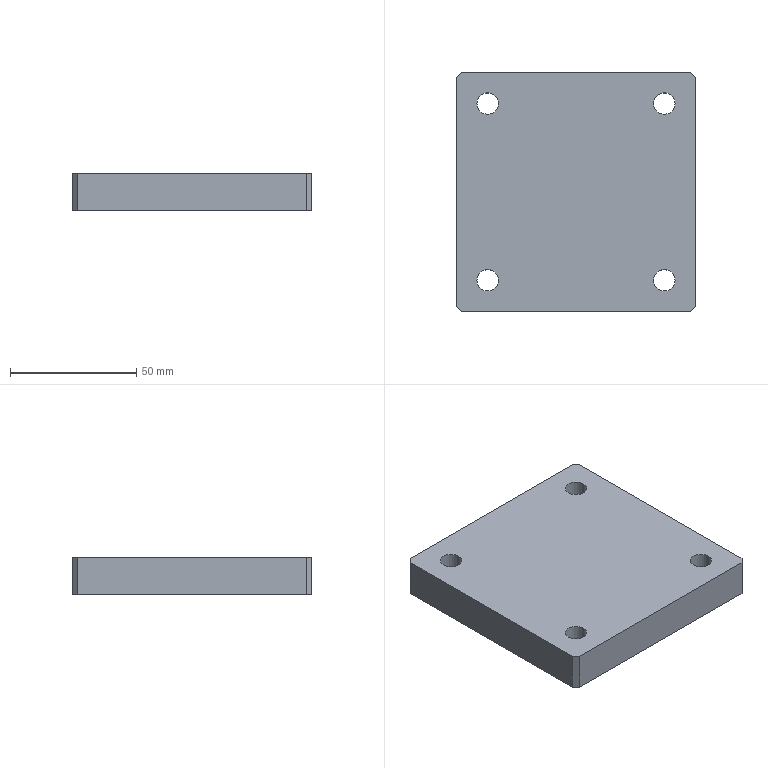Part | STEP file | ASND-0110-E63-HLTP01-005 | 1 solid | 18 faces | box 95 x 95 x 15 mm | volume 131850 mm3 | plane 10 | cylinder 8 | commonest cylinder face diameters 8.5 x8
STEP:
#1=CARTESIAN_POINT('',(0.,0.,0.));
#2=DIRECTION('',(0.,0.,1.));
#3=DIRECTION('',(1.,0.,0.));
#4=AXIS2_PLACEMENT_3D('',#1,#2,#3);
#5=CARTESIAN_POINT('',(16.75,82.5,0.));
#6=VERTEX_POINT('',#5);
#7=CARTESIAN_POINT('',(16.75,82.5,15.));
#8=VERTEX_POINT('',#7);
#9=CARTESIAN_POINT('',(16.75,82.5,15.));
#10=DIRECTION('',(0.,0.,1.));
#11=VECTOR('',#10,1.);
#12=LINE('',#9,#11);
#13=CARTESIAN_POINT('',(12.5,82.5,15.));
#14=DIRECTION('',(0.,0.,1.));
#15=DIRECTION('',(1.,0.,0.));
#16=AXIS2_PLACEMENT_3D('',#13,#14,#15);
#17=CYLINDRICAL_SURFACE('',#16,4.25);
#18=CARTESIAN_POINT('',(6.283,0.));
#19=DIRECTION('',(0.,1.));
#20=VECTOR('',#19,1.);
#21=LINE('',#18,#20);
#22=(GEOMETRIC_REPRESENTATION_CONTEXT(2)PARAMETRIC_REPRESENTATION_CONTEXT()REPRESENTATION_CONTEXT('',''));
#23=DEFINITIONAL_REPRESENTATION('',(#21),#22);
#24=PCURVE('',#17,#23);
#25=CARTESIAN_POINT('',(12.5,82.5,15.));
#26=DIRECTION('',(0.,0.,1.));
#27=DIRECTION('',(1.,0.,0.));
#28=AXIS2_PLACEMENT_3D('',#25,#26,#27);
#29=CYLINDRICAL_SURFACE('',#28,4.25);
#30=CARTESIAN_POINT('',(0.,0.));
#31=DIRECTION('',(0.,1.));
#32=VECTOR('',#31,1.);
#33=LINE('',#30,#32);
#34=(GEOMETRIC_REPRESENTATION_CONTEXT(2)PARAMETRIC_REPRESENTATION_CONTEXT()REPRESENTATION_CONTEXT('',''));
#35=DEFINITIONAL_REPRESENTATION('',(#33),#34);
#36=PCURVE('',#29,#35);
#37=SURFACE_CURVE('',#12,(#24,#36),.PCURVE_S1.);
#38=EDGE_CURVE('',#6,#8,#37,.T.);
#39=ORIENTED_EDGE('',*,*,#38,.T.);
#40=CARTESIAN_POINT('',(8.25,82.5,15.));
#41=VERTEX_POINT('',#40);
#42=CARTESIAN_POINT('',(12.5,82.5,15.));
#43=DIRECTION('',(0.,0.,1.));
#44=DIRECTION('',(1.,0.,0.));
#45=AXIS2_PLACEMENT_3D('',#42,#43,#44);
#46=CIRCLE('',#45,4.25);
#47=CARTESIAN_POINT('',(0.,0.));
#48=DIRECTION('',(1.,0.));
#49=VECTOR('',#48,1.);
#50=LINE('',#47,#49);
#51=(GEOMETRIC_REPRESENTATION_CONTEXT(2)PARAMETRIC_REPRESENTATION_CONTEXT()REPRESENTATION_CONTEXT('',''));
#52=DEFINITIONAL_REPRESENTATION('',(#50),#51);
#53=PCURVE('',#17,#52);
#54=CARTESIAN_POINT('',(45.,45.,15.));
#55=DIRECTION('',(0.,0.,1.));
#56=DIRECTION('',(0.7071,0.7071,0.));
#57=AXIS2_PLACEMENT_3D('',#54,#55,#56);
#58=PLANE('',#57);
#59=CARTESIAN_POINT('',(3.536,49.497));
#60=DIRECTION('',(0.7071,-0.7071));
#61=AXIS2_PLACEMENT_2D('',#59,#60);
#62=CIRCLE('',#61,4.25);
#63=(GEOMETRIC_REPRESENTATION_CONTEXT(2)PARAMETRIC_REPRESENTATION_CONTEXT()REPRESENTATION_CONTEXT('',''));
#64=DEFINITIONAL_REPRESENTATION('',(#62),#63);
#65=PCURVE('',#58,#64);
#66=SURFACE_CURVE('',#46,(#53,#65),.PCURVE_S1.);
#67=EDGE_CURVE('',#41,#8,#66,.T.);
#68=ORIENTED_EDGE('',*,*,#67,.F.);
#69=CARTESIAN_POINT('',(8.25,82.5,0.));
#70=VERTEX_POINT('',#69);
#71=CARTESIAN_POINT('',(8.25,82.5,15.));
#72=DIRECTION('',(0.,0.,1.));
#73=VECTOR('',#72,1.);
#74=LINE('',#71,#73);
#75=CARTESIAN_POINT('',(3.142,0.));
#76=DIRECTION('',(0.,1.));
#77=VECTOR('',#76,1.);
#78=LINE('',#75,#77);
#79=(GEOMETRIC_REPRESENTATION_CONTEXT(2)PARAMETRIC_REPRESENTATION_CONTEXT()REPRESENTATION_CONTEXT('',''));
#80=DEFINITIONAL_REPRESENTATION('',(#78),#79);
#81=PCURVE('',#17,#80);
#82=CARTESIAN_POINT('',(3.142,0.));
#83=DIRECTION('',(0.,1.));
#84=VECTOR('',#83,1.);
#85=LINE('',#82,#84);
#86=(GEOMETRIC_REPRESENTATION_CONTEXT(2)PARAMETRIC_REPRESENTATION_CONTEXT()REPRESENTATION_CONTEXT('',''));
#87=DEFINITIONAL_REPRESENTATION('',(#85),#86);
#88=PCURVE('',#29,#87);
#89=SURFACE_CURVE('',#74,(#81,#88),.PCURVE_S1.);
#90=EDGE_CURVE('',#70,#41,#89,.T.);
#91=ORIENTED_EDGE('',*,*,#90,.F.);
#92=CARTESIAN_POINT('',(12.5,82.5,0.));
#93=DIRECTION('',(0.,0.,1.));
#94=DIRECTION('',(1.,0.,0.));
#95=AXIS2_PLACEMENT_3D('',#92,#93,#94);
#96=CIRCLE('',#95,4.25);
#97=CARTESIAN_POINT('',(0.,-15.));
#98=DIRECTION('',(1.,0.));
#99=VECTOR('',#98,1.);
#100=LINE('',#97,#99);
#101=(GEOMETRIC_REPRESENTATION_CONTEXT(2)PARAMETRIC_REPRESENTATION_CONTEXT()REPRESENTATION_CONTEXT('',''));
#102=DEFINITIONAL_REPRESENTATION('',(#100),#101);
#103=PCURVE('',#17,#102);
#104=CARTESIAN_POINT('',(45.,45.,0.));
#105=DIRECTION('',(0.,0.,1.));
#106=DIRECTION('',(0.7071,0.7071,0.));
#107=AXIS2_PLACEMENT_3D('',#104,#105,#106);
#108=PLANE('',#107);
#109=CARTESIAN_POINT('',(3.536,49.497));
#110=DIRECTION('',(0.7071,-0.7071));
#111=AXIS2_PLACEMENT_2D('',#109,#110);
#112=CIRCLE('',#111,4.25);
#113=(GEOMETRIC_REPRESENTATION_CONTEXT(2)PARAMETRIC_REPRESENTATION_CONTEXT()REPRESENTATION_CONTEXT('',''));
#114=DEFINITIONAL_REPRESENTATION('',(#112),#113);
#115=PCURVE('',#108,#114);
#116=SURFACE_CURVE('',#96,(#103,#115),.PCURVE_S1.);
#117=EDGE_CURVE('',#70,#6,#116,.T.);
#118=ORIENTED_EDGE('',*,*,#117,.T.);
#119=EDGE_LOOP('',(#39,#68,#91,#118));
#120=FACE_BOUND('',#119,.F.);
#121=ADVANCED_FACE('',(#120),#17,.F.);
#122=CARTESIAN_POINT('',(86.75,82.5,0.));
#123=VERTEX_POINT('',#122);
#124=CARTESIAN_POINT('',(86.75,82.5,15.));
#125=VERTEX_POINT('',#124);
#126=CARTESIAN_POINT('',(86.75,82.5,15.));
#127=DIRECTION('',(0.,0.,1.));
#128=VECTOR('',#127,1.);
#129=LINE('',#126,#128);
#130=CARTESIAN_POINT('',(82.5,82.5,15.));
#131=DIRECTION('',(0.,0.,1.));
#132=DIRECTION('',(1.,0.,0.));
#133=AXIS2_PLACEMENT_3D('',#130,#131,#132);
#134=CYLINDRICAL_SURFACE('',#133,4.25);
#135=CARTESIAN_POINT('',(6.283,0.));
#136=DIRECTION('',(0.,1.));
#137=VECTOR('',#136,1.);
#138=LINE('',#135,#137);
#139=(GEOMETRIC_REPRESENTATION_CONTEXT(2)PARAMETRIC_REPRESENTATION_CONTEXT()REPRESENTATION_CONTEXT('',''));
#140=DEFINITIONAL_REPRESENTATION('',(#138),#139);
#141=PCURVE('',#134,#140);
#142=CARTESIAN_POINT('',(82.5,82.5,15.));
#143=DIRECTION('',(0.,0.,1.));
#144=DIRECTION('',(1.,0.,0.));
#145=AXIS2_PLACEMENT_3D('',#142,#143,#144);
#146=CYLINDRICAL_SURFACE('',#145,4.25);
#147=CARTESIAN_POINT('',(0.,0.));
#148=DIRECTION('',(0.,1.));
#149=VECTOR('',#148,1.);
#150=LINE('',#147,#149);
#151=(GEOMETRIC_REPRESENTATION_CONTEXT(2)PARAMETRIC_REPRESENTATION_CONTEXT()REPRESENTATION_CONTEXT('',''));
#152=DEFINITIONAL_REPRESENTATION('',(#150),#151);
#153=PCURVE('',#146,#152);
#154=SURFACE_CURVE('',#129,(#141,#153),.PCURVE_S1.);
#155=EDGE_CURVE('',#123,#125,#154,.T.);
#156=ORIENTED_EDGE('',*,*,#155,.T.);
#157=CARTESIAN_POINT('',(78.25,82.5,15.));
#158=VERTEX_POINT('',#157);
#159=CARTESIAN_POINT('',(82.5,82.5,15.));
#160=DIRECTION('',(0.,0.,1.));
#161=DIRECTION('',(1.,0.,0.));
#162=AXIS2_PLACEMENT_3D('',#159,#160,#161);
#163=CIRCLE('',#162,4.25);
#164=CARTESIAN_POINT('',(0.,0.));
#165=DIRECTION('',(1.,0.));
#166=VECTOR('',#165,1.);
#167=LINE('',#164,#166);
#168=(GEOMETRIC_REPRESENTATION_CONTEXT(2)PARAMETRIC_REPRESENTATION_CONTEXT()REPRESENTATION_CONTEXT('',''));
#169=DEFINITIONAL_REPRESENTATION('',(#167),#168);
#170=PCURVE('',#134,#169);
#171=CARTESIAN_POINT('',(53.033,0.));
#172=DIRECTION('',(0.7071,-0.7071));
#173=AXIS2_PLACEMENT_2D('',#171,#172);
#174=CIRCLE('',#173,4.25);
#175=(GEOMETRIC_REPRESENTATION_CONTEXT(2)PARAMETRIC_REPRESENTATION_CONTEXT()REPRESENTATION_CONTEXT('',''));
#176=DEFINITIONAL_REPRESENTATION('',(#174),#175);
#177=PCURVE('',#58,#176);
#178=SURFACE_CURVE('',#163,(#170,#177),.PCURVE_S1.);
#179=EDGE_CURVE('',#158,#125,#178,.T.);
#180=ORIENTED_EDGE('',*,*,#179,.F.);
#181=CARTESIAN_POINT('',(78.25,82.5,0.));
#182=VERTEX_POINT('',#181);
#183=CARTESIAN_POINT('',(78.25,82.5,15.));
#184=DIRECTION('',(0.,0.,1.));
#185=VECTOR('',#184,1.);
#186=LINE('',#183,#185);
#187=CARTESIAN_POINT('',(3.142,0.));
#188=DIRECTION('',(0.,1.));
#189=VECTOR('',#188,1.);
#190=LINE('',#187,#189);
#191=(GEOMETRIC_REPRESENTATION_CONTEXT(2)PARAMETRIC_REPRESENTATION_CONTEXT()REPRESENTATION_CONTEXT('',''));
#192=DEFINITIONAL_REPRESENTATION('',(#190),#191);
#193=PCURVE('',#134,#192);
#194=CARTESIAN_POINT('',(3.142,0.));
#195=DIRECTION('',(0.,1.));
#196=VECTOR('',#195,1.);
#197=LINE('',#194,#196);
#198=(GEOMETRIC_REPRESENTATION_CONTEXT(2)PARAMETRIC_REPRESENTATION_CONTEXT()REPRESENTATION_CONTEXT('',''));
#199=DEFINITIONAL_REPRESENTATION('',(#197),#198);
#200=PCURVE('',#146,#199);
#201=SURFACE_CURVE('',#186,(#193,#200),.PCURVE_S1.);
#202=EDGE_CURVE('',#182,#158,#201,.T.);
#203=ORIENTED_EDGE('',*,*,#202,.F.);
#204=CARTESIAN_POINT('',(82.5,82.5,0.));
#205=DIRECTION('',(0.,0.,1.));
#206=DIRECTION('',(1.,0.,0.));
#207=AXIS2_PLACEMENT_3D('',#204,#205,#206);
#208=CIRCLE('',#207,4.25);
#209=CARTESIAN_POINT('',(0.,-15.));
#210=DIRECTION('',(1.,0.));
#211=VECTOR('',#210,1.);
#212=LINE('',#209,#211);
#213=(GEOMETRIC_REPRESENTATION_CONTEXT(2)PARAMETRIC_REPRESENTATION_CONTEXT()REPRESENTATION_CONTEXT('',''));
#214=DEFINITIONAL_REPRESENTATION('',(#212),#213);
#215=PCURVE('',#134,#214);
#216=CARTESIAN_POINT('',(53.033,0.));
#217=DIRECTION('',(0.7071,-0.7071));
#218=AXIS2_PLACEMENT_2D('',#216,#217);
#219=CIRCLE('',#218,4.25);
#220=(GEOMETRIC_REPRESENTATION_CONTEXT(2)PARAMETRIC_REPRESENTATION_CONTEXT()REPRESENTATION_CONTEXT('',''));
#221=DEFINITIONAL_REPRESENTATION('',(#219),#220);
#222=PCURVE('',#108,#221);
#223=SURFACE_CURVE('',#208,(#215,#222),.PCURVE_S1.);
#224=EDGE_CURVE('',#182,#123,#223,.T.);
#225=ORIENTED_EDGE('',*,*,#224,.T.);
#226=EDGE_LOOP('',(#156,#180,#203,#225));
#227=FACE_BOUND('',#226,.F.);
#228=ADVANCED_FACE('',(#227),#134,.F.);
#229=CARTESIAN_POINT('',(86.75,12.5,0.));
#230=VERTEX_POINT('',#229);
#231=CARTESIAN_POINT('',(86.75,12.5,15.));
#232=VERTEX_POINT('',#231);
#233=CARTESIAN_POINT('',(86.75,12.5,15.));
#234=DIRECTION('',(0.,0.,1.));
#235=VECTOR('',#234,1.);
#236=LINE('',#233,#235);
#237=CARTESIAN_POINT('',(82.5,12.5,15.));
#238=DIRECTION('',(0.,0.,1.));
#239=DIRECTION('',(1.,0.,0.));
#240=AXIS2_PLACEMENT_3D('',#237,#238,#239);
#241=CYLINDRICAL_SURFACE('',#240,4.25);
#242=CARTESIAN_POINT('',(6.283,0.));
#243=DIRECTION('',(0.,1.));
#244=VECTOR('',#243,1.);
#245=LINE('',#242,#244);
#246=(GEOMETRIC_REPRESENTATION_CONTEXT(2)PARAMETRIC_REPRESENTATION_CONTEXT()REPRESENTATION_CONTEXT('',''));
#247=DEFINITIONAL_REPRESENTATION('',(#245),#246);
#248=PCURVE('',#241,#247);
#249=CARTESIAN_POINT('',(82.5,12.5,15.));
#250=DIRECTION('',(0.,0.,1.));
#251=DIRECTION('',(1.,0.,0.));
#252=AXIS2_PLACEMENT_3D('',#249,#250,#251);
#253=CYLINDRICAL_SURFACE('',#252,4.25);
#254=CARTESIAN_POINT('',(0.,0.));
#255=DIRECTION('',(0.,1.));
#256=VECTOR('',#255,1.);
#257=LINE('',#254,#256);
#258=(GEOMETRIC_REPRESENTATION_CONTEXT(2)PARAMETRIC_REPRESENTATION_CONTEXT()REPRESENTATION_CONTEXT('',''));
#259=DEFINITIONAL_REPRESENTATION('',(#257),#258);
#260=PCURVE('',#253,#259);
#261=SURFACE_CURVE('',#236,(#248,#260),.PCURVE_S1.);
#262=EDGE_CURVE('',#230,#232,#261,.T.);
#263=ORIENTED_EDGE('',*,*,#262,.T.);
#264=CARTESIAN_POINT('',(78.25,12.5,15.));
#265=VERTEX_POINT('',#264);
#266=CARTESIAN_POINT('',(82.5,12.5,15.));
#267=DIRECTION('',(0.,0.,1.));
#268=DIRECTION('',(1.,0.,0.));
#269=AXIS2_PLACEMENT_3D('',#266,#267,#268);
#270=CIRCLE('',#269,4.25);
#271=CARTESIAN_POINT('',(0.,0.));
#272=DIRECTION('',(1.,0.));
#273=VECTOR('',#272,1.);
#274=LINE('',#271,#273);
#275=(GEOMETRIC_REPRESENTATION_CONTEXT(2)PARAMETRIC_REPRESENTATION_CONTEXT()REPRESENTATION_CONTEXT('',''));
#276=DEFINITIONAL_REPRESENTATION('',(#274),#275);
#277=PCURVE('',#241,#276);
#278=CARTESIAN_POINT('',(3.536,-49.497));
#279=DIRECTION('',(0.7071,-0.7071));
#280=AXIS2_PLACEMENT_2D('',#278,#279);
#281=CIRCLE('',#280,4.25);
#282=(GEOMETRIC_REPRESENTATION_CONTEXT(2)PARAMETRIC_REPRESENTATION_CONTEXT()REPRESENTATION_CONTEXT('',''));
#283=DEFINITIONAL_REPRESENTATION('',(#281),#282);
#284=PCURVE('',#58,#283);
#285=SURFACE_CURVE('',#270,(#277,#284),.PCURVE_S1.);
#286=EDGE_CURVE('',#265,#232,#285,.T.);
#287=ORIENTED_EDGE('',*,*,#286,.F.);
#288=CARTESIAN_POINT('',(78.25,12.5,0.));
#289=VERTEX_POINT('',#288);
#290=CARTESIAN_POINT('',(78.25,12.5,15.));
#291=DIRECTION('',(0.,0.,1.));
#292=VECTOR('',#291,1.);
#293=LINE('',#290,#292);
#294=CARTESIAN_POINT('',(3.142,0.));
#295=DIRECTION('',(0.,1.));
#296=VECTOR('',#295,1.);
#297=LINE('',#294,#296);
#298=(GEOMETRIC_REPRESENTATION_CONTEXT(2)PARAMETRIC_REPRESENTATION_CONTEXT()REPRESENTATION_CONTEXT('',''));
#299=DEFINITIONAL_REPRESENTATION('',(#297),#298);
#300=PCURVE('',#241,#299);
#301=CARTESIAN_POINT('',(3.142,0.));
#302=DIRECTION('',(0.,1.));
#303=VECTOR('',#302,1.);
#304=LINE('',#301,#303);
#305=(GEOMETRIC_REPRESENTATION_CONTEXT(2)PARAMETRIC_REPRESENTATION_CONTEXT()REPRESENTATION_CONTEXT('',''));
#306=DEFINITIONAL_REPRESENTATION('',(#304),#305);
#307=PCURVE('',#253,#306);
#308=SURFACE_CURVE('',#293,(#300,#307),.PCURVE_S1.);
#309=EDGE_CURVE('',#289,#265,#308,.T.);
#310=ORIENTED_EDGE('',*,*,#309,.F.);
#311=CARTESIAN_POINT('',(82.5,12.5,0.));
#312=DIRECTION('',(0.,0.,1.));
#313=DIRECTION('',(1.,0.,0.));
#314=AXIS2_PLACEMENT_3D('',#311,#312,#313);
#315=CIRCLE('',#314,4.25);
#316=CARTESIAN_POINT('',(0.,-15.));
#317=DIRECTION('',(1.,0.));
#318=VECTOR('',#317,1.);
#319=LINE('',#316,#318);
#320=(GEOMETRIC_REPRESENTATION_CONTEXT(2)PARAMETRIC_REPRESENTATION_CONTEXT()REPRESENTATION_CONTEXT('',''));
#321=DEFINITIONAL_REPRESENTATION('',(#319),#320);
#322=PCURVE('',#241,#321);
#323=CARTESIAN_POINT('',(3.536,-49.497));
#324=DIRECTION('',(0.7071,-0.7071));
#325=AXIS2_PLACEMENT_2D('',#323,#324);
#326=CIRCLE('',#325,4.25);
#327=(GEOMETRIC_REPRESENTATION_CONTEXT(2)PARAMETRIC_REPRESENTATION_CONTEXT()REPRESENTATION_CONTEXT('',''));
#328=DEFINITIONAL_REPRESENTATION('',(#326),#327);
#329=PCURVE('',#108,#328);
#330=SURFACE_CURVE('',#315,(#322,#329),.PCURVE_S1.);
#331=EDGE_CURVE('',#289,#230,#330,.T.);
#332=ORIENTED_EDGE('',*,*,#331,.T.);
#333=EDGE_LOOP('',(#263,#287,#310,#332));
#334=FACE_BOUND('',#333,.F.);
#335=ADVANCED_FACE('',(#334),#241,.F.);
#336=CARTESIAN_POINT('',(16.75,12.5,0.));
#337=VERTEX_POINT('',#336);
#338=CARTESIAN_POINT('',(16.75,12.5,15.));
#339=VERTEX_POINT('',#338);
#340=CARTESIAN_POINT('',(16.75,12.5,15.));
#341=DIRECTION('',(0.,0.,1.));
#342=VECTOR('',#341,1.);
#343=LINE('',#340,#342);
#344=CARTESIAN_POINT('',(12.5,12.5,15.));
#345=DIRECTION('',(0.,0.,1.));
#346=DIRECTION('',(1.,0.,0.));
#347=AXIS2_PLACEMENT_3D('',#344,#345,#346);
#348=CYLINDRICAL_SURFACE('',#347,4.25);
#349=CARTESIAN_POINT('',(6.283,0.));
#350=DIRECTION('',(0.,1.));
#351=VECTOR('',#350,1.);
#352=LINE('',#349,#351);
#353=(GEOMETRIC_REPRESENTATION_CONTEXT(2)PARAMETRIC_REPRESENTATION_CONTEXT()REPRESENTATION_CONTEXT('',''));
#354=DEFINITIONAL_REPRESENTATION('',(#352),#353);
#355=PCURVE('',#348,#354);
#356=CARTESIAN_POINT('',(12.5,12.5,15.));
#357=DIRECTION('',(0.,0.,1.));
#358=DIRECTION('',(1.,0.,0.));
#359=AXIS2_PLACEMENT_3D('',#356,#357,#358);
#360=CYLINDRICAL_SURFACE('',#359,4.25);
#361=CARTESIAN_POINT('',(0.,0.));
#362=DIRECTION('',(0.,1.));
#363=VECTOR('',#362,1.);
#364=LINE('',#361,#363);
#365=(GEOMETRIC_REPRESENTATION_CONTEXT(2)PARAMETRIC_REPRESENTATION_CONTEXT()REPRESENTATION_CONTEXT('',''));
#366=DEFINITIONAL_REPRESENTATION('',(#364),#365);
#367=PCURVE('',#360,#366);
#368=SURFACE_CURVE('',#343,(#355,#367),.PCURVE_S1.);
#369=EDGE_CURVE('',#337,#339,#368,.T.);
#370=ORIENTED_EDGE('',*,*,#369,.T.);
#371=CARTESIAN_POINT('',(8.25,12.5,15.));
#372=VERTEX_POINT('',#371);
#373=CARTESIAN_POINT('',(12.5,12.5,15.));
#374=DIRECTION('',(0.,0.,1.));
#375=DIRECTION('',(1.,0.,0.));
#376=AXIS2_PLACEMENT_3D('',#373,#374,#375);
#377=CIRCLE('',#376,4.25);
#378=CARTESIAN_POINT('',(0.,0.));
#379=DIRECTION('',(1.,0.));
#380=VECTOR('',#379,1.);
#381=LINE('',#378,#380);
#382=(GEOMETRIC_REPRESENTATION_CONTEXT(2)PARAMETRIC_REPRESENTATION_CONTEXT()REPRESENTATION_CONTEXT('',''));
#383=DEFINITIONAL_REPRESENTATION('',(#381),#382);
#384=PCURVE('',#348,#383);
#385=CARTESIAN_POINT('',(-45.962,0.));
#386=DIRECTION('',(0.7071,-0.7071));
#387=AXIS2_PLACEMENT_2D('',#385,#386);
#388=CIRCLE('',#387,4.25);
#389=(GEOMETRIC_REPRESENTATION_CONTEXT(2)PARAMETRIC_REPRESENTATION_CONTEXT()REPRESENTATION_CONTEXT('',''));
#390=DEFINITIONAL_REPRESENTATION('',(#388),#389);
#391=PCURVE('',#58,#390);
#392=SURFACE_CURVE('',#377,(#384,#391),.PCURVE_S1.);
#393=EDGE_CURVE('',#372,#339,#392,.T.);
#394=ORIENTED_EDGE('',*,*,#393,.F.);
#395=CARTESIAN_POINT('',(8.25,12.5,0.));
#396=VERTEX_POINT('',#395);
#397=CARTESIAN_POINT('',(8.25,12.5,15.));
#398=DIRECTION('',(0.,0.,1.));
#399=VECTOR('',#398,1.);
#400=LINE('',#397,#399);
#401=CARTESIAN_POINT('',(3.142,0.));
#402=DIRECTION('',(0.,1.));
#403=VECTOR('',#402,1.);
#404=LINE('',#401,#403);
#405=(GEOMETRIC_REPRESENTATION_CONTEXT(2)PARAMETRIC_REPRESENTATION_CONTEXT()REPRESENTATION_CONTEXT('',''));
#406=DEFINITIONAL_REPRESENTATION('',(#404),#405);
#407=PCURVE('',#348,#406);
#408=CARTESIAN_POINT('',(3.142,0.));
#409=DIRECTION('',(0.,1.));
#410=VECTOR('',#409,1.);
#411=LINE('',#408,#410);
#412=(GEOMETRIC_REPRESENTATION_CONTEXT(2)PARAMETRIC_REPRESENTATION_CONTEXT()REPRESENTATION_CONTEXT('',''));
#413=DEFINITIONAL_REPRESENTATION('',(#411),#412);
#414=PCURVE('',#360,#413);
#415=SURFACE_CURVE('',#400,(#407,#414),.PCURVE_S1.);
#416=EDGE_CURVE('',#396,#372,#415,.T.);
#417=ORIENTED_EDGE('',*,*,#416,.F.);
#418=CARTESIAN_POINT('',(12.5,12.5,0.));
#419=DIRECTION('',(0.,0.,1.));
#420=DIRECTION('',(1.,0.,0.));
#421=AXIS2_PLACEMENT_3D('',#418,#419,#420);
#422=CIRCLE('',#421,4.25);
#423=CARTESIAN_POINT('',(0.,-15.));
#424=DIRECTION('',(1.,0.));
#425=VECTOR('',#424,1.);
#426=LINE('',#423,#425);
#427=(GEOMETRIC_REPRESENTATION_CONTEXT(2)PARAMETRIC_REPRESENTATION_CONTEXT()REPRESENTATION_CONTEXT('',''));
#428=DEFINITIONAL_REPRESENTATION('',(#426),#427);
#429=PCURVE('',#348,#428);
#430=CARTESIAN_POINT('',(-45.962,0.));
#431=DIRECTION('',(0.7071,-0.7071));
#432=AXIS2_PLACEMENT_2D('',#430,#431);
#433=CIRCLE('',#432,4.25);
#434=(GEOMETRIC_REPRESENTATION_CONTEXT(2)PARAMETRIC_REPRESENTATION_CONTEXT()REPRESENTATION_CONTEXT('',''));
#435=DEFINITIONAL_REPRESENTATION('',(#433),#434);
#436=PCURVE('',#108,#435);
#437=SURFACE_CURVE('',#422,(#429,#436),.PCURVE_S1.);
#438=EDGE_CURVE('',#396,#337,#437,.T.);
#439=ORIENTED_EDGE('',*,*,#438,.T.);
#440=EDGE_LOOP('',(#370,#394,#417,#439));
#441=FACE_BOUND('',#440,.F.);
#442=ADVANCED_FACE('',(#441),#348,.F.);
#443=CARTESIAN_POINT('',(0.,2.,15.));
#444=VERTEX_POINT('',#443);
#445=CARTESIAN_POINT('',(0.,93.,15.));
#446=VERTEX_POINT('',#445);
#447=CARTESIAN_POINT('',(0.,2.,15.));
#448=DIRECTION('',(0.,1.,0.));
#449=VECTOR('',#448,1.);
#450=LINE('',#447,#449);
#451=CARTESIAN_POINT('',(0.,0.,0.));
#452=DIRECTION('',(-1.,0.,0.));
#453=DIRECTION('',(0.,0.7071,0.7071));
#454=AXIS2_PLACEMENT_3D('',#451,#452,#453);
#455=PLANE('',#454);
#456=CARTESIAN_POINT('',(12.021,-9.192));
#457=DIRECTION('',(0.7071,0.7071));
#458=VECTOR('',#457,1.);
#459=LINE('',#456,#458);
#460=(GEOMETRIC_REPRESENTATION_CONTEXT(2)PARAMETRIC_REPRESENTATION_CONTEXT()REPRESENTATION_CONTEXT('',''));
#461=DEFINITIONAL_REPRESENTATION('',(#459),#460);
#462=PCURVE('',#455,#461);
#463=CARTESIAN_POINT('',(-62.225,1.414));
#464=DIRECTION('',(0.7071,0.7071));
#465=VECTOR('',#464,1.);
#466=LINE('',#463,#465);
#467=(GEOMETRIC_REPRESENTATION_CONTEXT(2)PARAMETRIC_REPRESENTATION_CONTEXT()REPRESENTATION_CONTEXT('',''));
#468=DEFINITIONAL_REPRESENTATION('',(#466),#467);
#469=PCURVE('',#58,#468);
#470=SURFACE_CURVE('',#450,(#462,#469),.PCURVE_S1.);
#471=EDGE_CURVE('',#444,#446,#470,.T.);
#472=ORIENTED_EDGE('',*,*,#471,.T.);
#473=CARTESIAN_POINT('',(0.,93.,0.));
#474=VERTEX_POINT('',#473);
#475=CARTESIAN_POINT('',(0.,93.,15.));
#476=DIRECTION('',(0.,0.,-1.));
#477=VECTOR('',#476,1.);
#478=LINE('',#475,#477);
#479=CARTESIAN_POINT('',(76.368,55.154));
#480=DIRECTION('',(-0.7071,0.7071));
#481=VECTOR('',#480,1.);
#482=LINE('',#479,#481);
#483=(GEOMETRIC_REPRESENTATION_CONTEXT(2)PARAMETRIC_REPRESENTATION_CONTEXT()REPRESENTATION_CONTEXT('',''));
#484=DEFINITIONAL_REPRESENTATION('',(#482),#483);
#485=PCURVE('',#455,#484);
#486=CARTESIAN_POINT('',(0.,93.,0.));
#487=DIRECTION('',(0.7071,-0.7071,0.));
#488=DIRECTION('',(0.5774,0.5774,0.5774));
#489=AXIS2_PLACEMENT_3D('',#486,#487,#488);
#490=PLANE('',#489);
#491=CARTESIAN_POINT('',(8.66,12.247));
#492=DIRECTION('',(-0.5774,-0.8165));
#493=VECTOR('',#492,1.);
#494=LINE('',#491,#493);
#495=(GEOMETRIC_REPRESENTATION_CONTEXT(2)PARAMETRIC_REPRESENTATION_CONTEXT()REPRESENTATION_CONTEXT('',''));
#496=DEFINITIONAL_REPRESENTATION('',(#494),#495);
#497=PCURVE('',#490,#496);
#498=SURFACE_CURVE('',#478,(#485,#497),.PCURVE_S1.);
#499=EDGE_CURVE('',#446,#474,#498,.T.);
#500=ORIENTED_EDGE('',*,*,#499,.T.);
#501=CARTESIAN_POINT('',(0.,2.,0.));
#502=VERTEX_POINT('',#501);
#503=CARTESIAN_POINT('',(0.,93.,0.));
#504=DIRECTION('',(0.,-1.,0.));
#505=VECTOR('',#504,1.);
#506=LINE('',#503,#505);
#507=CARTESIAN_POINT('',(65.761,65.761));
#508=DIRECTION('',(-0.7071,-0.7071));
#509=VECTOR('',#508,1.);
#510=LINE('',#507,#509);
#511=(GEOMETRIC_REPRESENTATION_CONTEXT(2)PARAMETRIC_REPRESENTATION_CONTEXT()REPRESENTATION_CONTEXT('',''));
#512=DEFINITIONAL_REPRESENTATION('',(#510),#511);
#513=PCURVE('',#455,#512);
#514=CARTESIAN_POINT('',(2.121,65.761));
#515=DIRECTION('',(-0.7071,-0.7071));
#516=VECTOR('',#515,1.);
#517=LINE('',#514,#516);
#518=(GEOMETRIC_REPRESENTATION_CONTEXT(2)PARAMETRIC_REPRESENTATION_CONTEXT()REPRESENTATION_CONTEXT('',''));
#519=DEFINITIONAL_REPRESENTATION('',(#517),#518);
#520=PCURVE('',#108,#519);
#521=SURFACE_CURVE('',#506,(#513,#520),.PCURVE_S1.);
#522=EDGE_CURVE('',#474,#502,#521,.T.);
#523=ORIENTED_EDGE('',*,*,#522,.T.);
#524=CARTESIAN_POINT('',(0.,2.,15.));
#525=DIRECTION('',(0.,0.,-1.));
#526=VECTOR('',#525,1.);
#527=LINE('',#524,#526);
#528=CARTESIAN_POINT('',(12.021,-9.192));
#529=DIRECTION('',(-0.7071,0.7071));
#530=VECTOR('',#529,1.);
#531=LINE('',#528,#530);
#532=(GEOMETRIC_REPRESENTATION_CONTEXT(2)PARAMETRIC_REPRESENTATION_CONTEXT()REPRESENTATION_CONTEXT('',''));
#533=DEFINITIONAL_REPRESENTATION('',(#531),#532);
#534=PCURVE('',#455,#533);
#535=CARTESIAN_POINT('',(1.,1.,0.));
#536=DIRECTION('',(-0.7071,-0.7071,0.));
#537=DIRECTION('',(-0.5774,0.5774,0.5774));
#538=AXIS2_PLACEMENT_3D('',#535,#536,#537);
#539=PLANE('',#538);
#540=CARTESIAN_POINT('',(9.815,-11.431));
#541=DIRECTION('',(-0.5774,0.8165));
#542=VECTOR('',#541,1.);
#543=LINE('',#540,#542);
#544=(GEOMETRIC_REPRESENTATION_CONTEXT(2)PARAMETRIC_REPRESENTATION_CONTEXT()REPRESENTATION_CONTEXT('',''));
#545=DEFINITIONAL_REPRESENTATION('',(#543),#544);
#546=PCURVE('',#539,#545);
#547=SURFACE_CURVE('',#527,(#534,#546),.PCURVE_S1.);
#548=EDGE_CURVE('',#444,#502,#547,.T.);
#549=ORIENTED_EDGE('',*,*,#548,.F.);
#550=EDGE_LOOP('',(#472,#500,#523,#549));
#551=FACE_BOUND('',#550,.T.);
#552=ADVANCED_FACE('',(#551),#455,.T.);
#553=ORIENTED_EDGE('',*,*,#522,.F.);
#554=CARTESIAN_POINT('',(2.,95.,0.));
#555=VERTEX_POINT('',#554);
#556=CARTESIAN_POINT('',(2.,95.,0.));
#557=DIRECTION('',(0.7071,0.7071,0.));
#558=VECTOR('',#557,1.);
#559=LINE('',#556,#558);
#560=CARTESIAN_POINT('',(4.95,65.761));
#561=DIRECTION('',(1.,0.));
#562=VECTOR('',#561,1.);
#563=LINE('',#560,#562);
#564=(GEOMETRIC_REPRESENTATION_CONTEXT(2)PARAMETRIC_REPRESENTATION_CONTEXT()REPRESENTATION_CONTEXT('',''));
#565=DEFINITIONAL_REPRESENTATION('',(#563),#564);
#566=PCURVE('',#108,#565);
#567=CARTESIAN_POINT('',(2.309,-1.633));
#568=DIRECTION('',(0.8165,-0.5774));
#569=VECTOR('',#568,1.);
#570=LINE('',#567,#569);
#571=(GEOMETRIC_REPRESENTATION_CONTEXT(2)PARAMETRIC_REPRESENTATION_CONTEXT()REPRESENTATION_CONTEXT('',''));
#572=DEFINITIONAL_REPRESENTATION('',(#570),#571);
#573=PCURVE('',#490,#572);
#574=SURFACE_CURVE('',#559,(#566,#573),.PCURVE_S1.);
#575=EDGE_CURVE('',#474,#555,#574,.T.);
#576=ORIENTED_EDGE('',*,*,#575,.T.);
#577=CARTESIAN_POINT('',(93.,95.,0.));
#578=VERTEX_POINT('',#577);
#579=CARTESIAN_POINT('',(2.,95.,0.));
#580=DIRECTION('',(1.,0.,0.));
#581=VECTOR('',#580,1.);
#582=LINE('',#579,#581);
#583=CARTESIAN_POINT('',(4.95,65.761));
#584=DIRECTION('',(0.7071,-0.7071));
#585=VECTOR('',#584,1.);
#586=LINE('',#583,#585);
#587=(GEOMETRIC_REPRESENTATION_CONTEXT(2)PARAMETRIC_REPRESENTATION_CONTEXT()REPRESENTATION_CONTEXT('',''));
#588=DEFINITIONAL_REPRESENTATION('',(#586),#587);
#589=PCURVE('',#108,#588);
#590=CARTESIAN_POINT('',(5.,95.,-127.279));
#591=DIRECTION('',(0.,1.,0.));
#592=DIRECTION('',(0.7071,0.,0.7071));
#593=AXIS2_PLACEMENT_3D('',#590,#591,#592);
#594=PLANE('',#593);
#595=CARTESIAN_POINT('',(87.879,-92.121));
#596=DIRECTION('',(0.7071,0.7071));
#597=VECTOR('',#596,1.);
#598=LINE('',#595,#597);
#599=(GEOMETRIC_REPRESENTATION_CONTEXT(2)PARAMETRIC_REPRESENTATION_CONTEXT()REPRESENTATION_CONTEXT('',''));
#600=DEFINITIONAL_REPRESENTATION('',(#598),#599);
#601=PCURVE('',#594,#600);
#602=SURFACE_CURVE('',#582,(#589,#601),.PCURVE_S1.);
#603=EDGE_CURVE('',#555,#578,#602,.T.);
#604=ORIENTED_EDGE('',*,*,#603,.T.);
#605=CARTESIAN_POINT('',(95.,93.,0.));
#606=VERTEX_POINT('',#605);
#607=CARTESIAN_POINT('',(95.,93.,0.));
#608=DIRECTION('',(0.7071,-0.7071,0.));
#609=VECTOR('',#608,1.);
#610=LINE('',#607,#609);
#611=CARTESIAN_POINT('',(69.296,-1.414));
#612=DIRECTION('',(0.,-1.));
#613=VECTOR('',#612,1.);
#614=LINE('',#611,#613);
#615=(GEOMETRIC_REPRESENTATION_CONTEXT(2)PARAMETRIC_REPRESENTATION_CONTEXT()REPRESENTATION_CONTEXT('',''));
#616=DEFINITIONAL_REPRESENTATION('',(#614),#615);
#617=PCURVE('',#108,#616);
#618=CARTESIAN_POINT('',(95.,93.,-127.279));
#619=DIRECTION('',(-0.7071,-0.7071,0.));
#620=DIRECTION('',(-0.5774,0.5774,0.5774));
#621=AXIS2_PLACEMENT_3D('',#618,#619,#620);
#622=PLANE('',#621);
#623=CARTESIAN_POINT('',(73.485,-103.923));
#624=DIRECTION('',(-0.8165,-0.5774));
#625=VECTOR('',#624,1.);
#626=LINE('',#623,#625);
#627=(GEOMETRIC_REPRESENTATION_CONTEXT(2)PARAMETRIC_REPRESENTATION_CONTEXT()REPRESENTATION_CONTEXT('',''));
#628=DEFINITIONAL_REPRESENTATION('',(#626),#627);
#629=PCURVE('',#622,#628);
#630=SURFACE_CURVE('',#610,(#617,#629),.PCURVE_S1.);
#631=EDGE_CURVE('',#578,#606,#630,.T.);
#632=ORIENTED_EDGE('',*,*,#631,.T.);
#633=CARTESIAN_POINT('',(95.,2.,0.));
#634=VERTEX_POINT('',#633);
#635=CARTESIAN_POINT('',(95.,93.,0.));
#636=DIRECTION('',(0.,-1.,0.));
#637=VECTOR('',#636,1.);
#638=LINE('',#635,#637);
#639=CARTESIAN_POINT('',(69.296,-1.414));
#640=DIRECTION('',(-0.7071,-0.7071));
#641=VECTOR('',#640,1.);
#642=LINE('',#639,#641);
#643=(GEOMETRIC_REPRESENTATION_CONTEXT(2)PARAMETRIC_REPRESENTATION_CONTEXT()REPRESENTATION_CONTEXT('',''));
#644=DEFINITIONAL_REPRESENTATION('',(#642),#643);
#645=PCURVE('',#108,#644);
#646=CARTESIAN_POINT('',(95.,5.,-127.279));
#647=DIRECTION('',(1.,0.,0.));
#648=DIRECTION('',(0.,0.7071,0.7071));
#649=AXIS2_PLACEMENT_3D('',#646,#647,#648);
#650=PLANE('',#649);
#651=CARTESIAN_POINT('',(152.225,27.775));
#652=DIRECTION('',(-0.7071,0.7071));
#653=VECTOR('',#652,1.);
#654=LINE('',#651,#653);
#655=(GEOMETRIC_REPRESENTATION_CONTEXT(2)PARAMETRIC_REPRESENTATION_CONTEXT()REPRESENTATION_CONTEXT('',''));
#656=DEFINITIONAL_REPRESENTATION('',(#654),#655);
#657=PCURVE('',#650,#656);
#658=SURFACE_CURVE('',#638,(#645,#657),.PCURVE_S1.);
#659=EDGE_CURVE('',#606,#634,#658,.T.);
#660=ORIENTED_EDGE('',*,*,#659,.T.);
#661=CARTESIAN_POINT('',(93.,0.,0.));
#662=VERTEX_POINT('',#661);
#663=CARTESIAN_POINT('',(93.,0.,0.));
#664=DIRECTION('',(-0.7071,-0.7071,0.));
#665=VECTOR('',#664,1.);
#666=LINE('',#663,#665);
#667=CARTESIAN_POINT('',(2.121,-65.761));
#668=DIRECTION('',(-1.,0.));
#669=VECTOR('',#668,1.);
#670=LINE('',#667,#669);
#671=(GEOMETRIC_REPRESENTATION_CONTEXT(2)PARAMETRIC_REPRESENTATION_CONTEXT()REPRESENTATION_CONTEXT('',''));
#672=DEFINITIONAL_REPRESENTATION('',(#670),#671);
#673=PCURVE('',#108,#672);
#674=CARTESIAN_POINT('',(95.,2.,-127.279));
#675=DIRECTION('',(-0.7071,0.7071,0.));
#676=DIRECTION('',(0.5774,0.5774,0.5774));
#677=AXIS2_PLACEMENT_3D('',#674,#675,#676);
#678=PLANE('',#677);
#679=CARTESIAN_POINT('',(71.175,-105.556));
#680=DIRECTION('',(-0.8165,-0.5774));
#681=VECTOR('',#680,1.);
#682=LINE('',#679,#681);
#683=(GEOMETRIC_REPRESENTATION_CONTEXT(2)PARAMETRIC_REPRESENTATION_CONTEXT()REPRESENTATION_CONTEXT('',''));
#684=DEFINITIONAL_REPRESENTATION('',(#682),#683);
#685=PCURVE('',#678,#684);
#686=SURFACE_CURVE('',#666,(#673,#685),.PCURVE_S1.);
#687=EDGE_CURVE('',#634,#662,#686,.T.);
#688=ORIENTED_EDGE('',*,*,#687,.T.);
#689=CARTESIAN_POINT('',(2.,0.,0.));
#690=VERTEX_POINT('',#689);
#691=CARTESIAN_POINT('',(2.,0.,0.));
#692=DIRECTION('',(1.,0.,0.));
#693=VECTOR('',#692,1.);
#694=LINE('',#691,#693);
#695=CARTESIAN_POINT('',(-62.225,-1.414));
#696=DIRECTION('',(0.7071,-0.7071));
#697=VECTOR('',#696,1.);
#698=LINE('',#695,#697);
#699=(GEOMETRIC_REPRESENTATION_CONTEXT(2)PARAMETRIC_REPRESENTATION_CONTEXT()REPRESENTATION_CONTEXT('',''));
#700=DEFINITIONAL_REPRESENTATION('',(#698),#699);
#701=PCURVE('',#108,#700);
#702=CARTESIAN_POINT('',(90.,0.,0.));
#703=DIRECTION('',(0.,-1.,0.));
#704=DIRECTION('',(0.7071,0.,0.7071));
#705=AXIS2_PLACEMENT_3D('',#702,#703,#704);
#706=PLANE('',#705);
#707=CARTESIAN_POINT('',(-62.225,62.225));
#708=DIRECTION('',(0.7071,-0.7071));
#709=VECTOR('',#708,1.);
#710=LINE('',#707,#709);
#711=(GEOMETRIC_REPRESENTATION_CONTEXT(2)PARAMETRIC_REPRESENTATION_CONTEXT()REPRESENTATION_CONTEXT('',''));
#712=DEFINITIONAL_REPRESENTATION('',(#710),#711);
#713=PCURVE('',#706,#712);
#714=SURFACE_CURVE('',#694,(#701,#713),.PCURVE_S1.);
#715=EDGE_CURVE('',#690,#662,#714,.T.);
#716=ORIENTED_EDGE('',*,*,#715,.F.);
#717=CARTESIAN_POINT('',(0.,2.,0.));
#718=DIRECTION('',(0.7071,-0.7071,0.));
#719=VECTOR('',#718,1.);
#720=LINE('',#717,#719);
#721=CARTESIAN_POINT('',(-62.225,1.414));
#722=DIRECTION('',(0.,-1.));
#723=VECTOR('',#722,1.);
#724=LINE('',#721,#723);
#725=(GEOMETRIC_REPRESENTATION_CONTEXT(2)PARAMETRIC_REPRESENTATION_CONTEXT()REPRESENTATION_CONTEXT('',''));
#726=DEFINITIONAL_REPRESENTATION('',(#724),#725);
#727=PCURVE('',#108,#726);
#728=CARTESIAN_POINT('',(1.155,0.8165));
#729=DIRECTION('',(-0.8165,-0.5774));
#730=VECTOR('',#729,1.);
#731=LINE('',#728,#730);
#732=(GEOMETRIC_REPRESENTATION_CONTEXT(2)PARAMETRIC_REPRESENTATION_CONTEXT()REPRESENTATION_CONTEXT('',''));
#733=DEFINITIONAL_REPRESENTATION('',(#731),#732);
#734=PCURVE('',#539,#733);
#735=SURFACE_CURVE('',#720,(#727,#734),.PCURVE_S1.);
#736=EDGE_CURVE('',#502,#690,#735,.T.);
#737=ORIENTED_EDGE('',*,*,#736,.F.);
#738=EDGE_LOOP('',(#553,#576,#604,#632,#660,#688,#716,#737));
#739=FACE_BOUND('',#738,.T.);
#740=CARTESIAN_POINT('',(12.5,82.5,0.));
#741=DIRECTION('',(0.,0.,1.));
#742=DIRECTION('',(1.,0.,0.));
#743=AXIS2_PLACEMENT_3D('',#740,#741,#742);
#744=CIRCLE('',#743,4.25);
#745=CARTESIAN_POINT('',(3.536,49.497));
#746=DIRECTION('',(0.7071,-0.7071));
#747=AXIS2_PLACEMENT_2D('',#745,#746);
#748=CIRCLE('',#747,4.25);
#749=(GEOMETRIC_REPRESENTATION_CONTEXT(2)PARAMETRIC_REPRESENTATION_CONTEXT()REPRESENTATION_CONTEXT('',''));
#750=DEFINITIONAL_REPRESENTATION('',(#748),#749);
#751=PCURVE('',#108,#750);
#752=CARTESIAN_POINT('',(0.,-15.));
#753=DIRECTION('',(1.,0.));
#754=VECTOR('',#753,1.);
#755=LINE('',#752,#754);
#756=(GEOMETRIC_REPRESENTATION_CONTEXT(2)PARAMETRIC_REPRESENTATION_CONTEXT()REPRESENTATION_CONTEXT('',''));
#757=DEFINITIONAL_REPRESENTATION('',(#755),#756);
#758=PCURVE('',#29,#757);
#759=SURFACE_CURVE('',#744,(#751,#758),.PCURVE_S1.);
#760=EDGE_CURVE('',#6,#70,#759,.T.);
#761=ORIENTED_EDGE('',*,*,#760,.T.);
#762=ORIENTED_EDGE('',*,*,#117,.T.);
#763=EDGE_LOOP('',(#761,#762));
#764=FACE_BOUND('',#763,.T.);
#765=CARTESIAN_POINT('',(82.5,82.5,0.));
#766=DIRECTION('',(0.,0.,1.));
#767=DIRECTION('',(1.,0.,0.));
#768=AXIS2_PLACEMENT_3D('',#765,#766,#767);
#769=CIRCLE('',#768,4.25);
#770=CARTESIAN_POINT('',(53.033,0.));
#771=DIRECTION('',(0.7071,-0.7071));
#772=AXIS2_PLACEMENT_2D('',#770,#771);
#773=CIRCLE('',#772,4.25);
#774=(GEOMETRIC_REPRESENTATION_CONTEXT(2)PARAMETRIC_REPRESENTATION_CONTEXT()REPRESENTATION_CONTEXT('',''));
#775=DEFINITIONAL_REPRESENTATION('',(#773),#774);
#776=PCURVE('',#108,#775);
#777=CARTESIAN_POINT('',(0.,-15.));
#778=DIRECTION('',(1.,0.));
#779=VECTOR('',#778,1.);
#780=LINE('',#777,#779);
#781=(GEOMETRIC_REPRESENTATION_CONTEXT(2)PARAMETRIC_REPRESENTATION_CONTEXT()REPRESENTATION_CONTEXT('',''));
#782=DEFINITIONAL_REPRESENTATION('',(#780),#781);
#783=PCURVE('',#146,#782);
#784=SURFACE_CURVE('',#769,(#776,#783),.PCURVE_S1.);
#785=EDGE_CURVE('',#123,#182,#784,.T.);
#786=ORIENTED_EDGE('',*,*,#785,.T.);
#787=ORIENTED_EDGE('',*,*,#224,.T.);
#788=EDGE_LOOP('',(#786,#787));
#789=FACE_BOUND('',#788,.T.);
#790=CARTESIAN_POINT('',(82.5,12.5,0.));
#791=DIRECTION('',(0.,0.,1.));
#792=DIRECTION('',(1.,0.,0.));
#793=AXIS2_PLACEMENT_3D('',#790,#791,#792);
#794=CIRCLE('',#793,4.25);
#795=CARTESIAN_POINT('',(3.536,-49.497));
#796=DIRECTION('',(0.7071,-0.7071));
#797=AXIS2_PLACEMENT_2D('',#795,#796);
#798=CIRCLE('',#797,4.25);
#799=(GEOMETRIC_REPRESENTATION_CONTEXT(2)PARAMETRIC_REPRESENTATION_CONTEXT()REPRESENTATION_CONTEXT('',''));
#800=DEFINITIONAL_REPRESENTATION('',(#798),#799);
#801=PCURVE('',#108,#800);
#802=CARTESIAN_POINT('',(0.,-15.));
#803=DIRECTION('',(1.,0.));
#804=VECTOR('',#803,1.);
#805=LINE('',#802,#804);
#806=(GEOMETRIC_REPRESENTATION_CONTEXT(2)PARAMETRIC_REPRESENTATION_CONTEXT()REPRESENTATION_CONTEXT('',''));
#807=DEFINITIONAL_REPRESENTATION('',(#805),#806);
#808=PCURVE('',#253,#807);
#809=SURFACE_CURVE('',#794,(#801,#808),.PCURVE_S1.);
#810=EDGE_CURVE('',#230,#289,#809,.T.);
#811=ORIENTED_EDGE('',*,*,#810,.T.);
#812=ORIENTED_EDGE('',*,*,#331,.T.);
#813=EDGE_LOOP('',(#811,#812));
#814=FACE_BOUND('',#813,.T.);
#815=CARTESIAN_POINT('',(12.5,12.5,0.));
#816=DIRECTION('',(0.,0.,1.));
#817=DIRECTION('',(1.,0.,0.));
#818=AXIS2_PLACEMENT_3D('',#815,#816,#817);
#819=CIRCLE('',#818,4.25);
#820=CARTESIAN_POINT('',(-45.962,0.));
#821=DIRECTION('',(0.7071,-0.7071));
#822=AXIS2_PLACEMENT_2D('',#820,#821);
#823=CIRCLE('',#822,4.25);
#824=(GEOMETRIC_REPRESENTATION_CONTEXT(2)PARAMETRIC_REPRESENTATION_CONTEXT()REPRESENTATION_CONTEXT('',''));
#825=DEFINITIONAL_REPRESENTATION('',(#823),#824);
#826=PCURVE('',#108,#825);
#827=CARTESIAN_POINT('',(0.,-15.));
#828=DIRECTION('',(1.,0.));
#829=VECTOR('',#828,1.);
#830=LINE('',#827,#829);
#831=(GEOMETRIC_REPRESENTATION_CONTEXT(2)PARAMETRIC_REPRESENTATION_CONTEXT()REPRESENTATION_CONTEXT('',''));
#832=DEFINITIONAL_REPRESENTATION('',(#830),#831);
#833=PCURVE('',#360,#832);
#834=SURFACE_CURVE('',#819,(#826,#833),.PCURVE_S1.);
#835=EDGE_CURVE('',#337,#396,#834,.T.);
#836=ORIENTED_EDGE('',*,*,#835,.T.);
#837=ORIENTED_EDGE('',*,*,#438,.T.);
#838=EDGE_LOOP('',(#836,#837));
#839=FACE_BOUND('',#838,.T.);
#840=ADVANCED_FACE('',(#739,#764,#789,#814,#839),#108,.F.);
#841=CARTESIAN_POINT('',(2.,0.,15.));
#842=VERTEX_POINT('',#841);
#843=CARTESIAN_POINT('',(2.,0.,15.));
#844=DIRECTION('',(-0.7071,0.7071,0.));
#845=VECTOR('',#844,1.);
#846=LINE('',#843,#845);
#847=CARTESIAN_POINT('',(7.506,-13.064));
#848=DIRECTION('',(0.8165,0.5774));
#849=VECTOR('',#848,1.);
#850=LINE('',#847,#849);
#851=(GEOMETRIC_REPRESENTATION_CONTEXT(2)PARAMETRIC_REPRESENTATION_CONTEXT()REPRESENTATION_CONTEXT('',''));
#852=DEFINITIONAL_REPRESENTATION('',(#850),#851);
#853=PCURVE('',#539,#852);
#854=CARTESIAN_POINT('',(-62.225,-1.414));
#855=DIRECTION('',(0.,1.));
#856=VECTOR('',#855,1.);
#857=LINE('',#854,#856);
#858=(GEOMETRIC_REPRESENTATION_CONTEXT(2)PARAMETRIC_REPRESENTATION_CONTEXT()REPRESENTATION_CONTEXT('',''));
#859=DEFINITIONAL_REPRESENTATION('',(#857),#858);
#860=PCURVE('',#58,#859);
#861=SURFACE_CURVE('',#846,(#853,#860),.PCURVE_S1.);
#862=EDGE_CURVE('',#842,#444,#861,.T.);
#863=ORIENTED_EDGE('',*,*,#862,.T.);
#864=ORIENTED_EDGE('',*,*,#548,.T.);
#865=ORIENTED_EDGE('',*,*,#736,.T.);
#866=CARTESIAN_POINT('',(2.,0.,0.));
#867=DIRECTION('',(0.,0.,1.));
#868=VECTOR('',#867,1.);
#869=LINE('',#866,#868);
#870=CARTESIAN_POINT('',(-1.155,-0.8165));
#871=DIRECTION('',(0.5774,-0.8165));
#872=VECTOR('',#871,1.);
#873=LINE('',#870,#872);
#874=(GEOMETRIC_REPRESENTATION_CONTEXT(2)PARAMETRIC_REPRESENTATION_CONTEXT()REPRESENTATION_CONTEXT('',''));
#875=DEFINITIONAL_REPRESENTATION('',(#873),#874);
#876=PCURVE('',#539,#875);
#877=CARTESIAN_POINT('',(-62.225,62.225));
#878=DIRECTION('',(0.7071,0.7071));
#879=VECTOR('',#878,1.);
#880=LINE('',#877,#879);
#881=(GEOMETRIC_REPRESENTATION_CONTEXT(2)PARAMETRIC_REPRESENTATION_CONTEXT()REPRESENTATION_CONTEXT('',''));
#882=DEFINITIONAL_REPRESENTATION('',(#880),#881);
#883=PCURVE('',#706,#882);
#884=SURFACE_CURVE('',#869,(#876,#883),.PCURVE_S1.);
#885=EDGE_CURVE('',#690,#842,#884,.T.);
#886=ORIENTED_EDGE('',*,*,#885,.T.);
#887=EDGE_LOOP('',(#863,#864,#865,#886));
#888=FACE_BOUND('',#887,.T.);
#889=ADVANCED_FACE('',(#888),#539,.T.);
#890=ORIENTED_EDGE('',*,*,#715,.T.);
#891=CARTESIAN_POINT('',(93.,0.,15.));
#892=VERTEX_POINT('',#891);
#893=CARTESIAN_POINT('',(93.,0.,0.));
#894=DIRECTION('',(0.,0.,1.));
#895=VECTOR('',#894,1.);
#896=LINE('',#893,#895);
#897=CARTESIAN_POINT('',(2.121,-2.121));
#898=DIRECTION('',(0.7071,0.7071));
#899=VECTOR('',#898,1.);
#900=LINE('',#897,#899);
#901=(GEOMETRIC_REPRESENTATION_CONTEXT(2)PARAMETRIC_REPRESENTATION_CONTEXT()REPRESENTATION_CONTEXT('',''));
#902=DEFINITIONAL_REPRESENTATION('',(#900),#901);
#903=PCURVE('',#706,#902);
#904=CARTESIAN_POINT('',(71.175,-105.556));
#905=DIRECTION('',(0.5774,-0.8165));
#906=VECTOR('',#905,1.);
#907=LINE('',#904,#906);
#908=(GEOMETRIC_REPRESENTATION_CONTEXT(2)PARAMETRIC_REPRESENTATION_CONTEXT()REPRESENTATION_CONTEXT('',''));
#909=DEFINITIONAL_REPRESENTATION('',(#907),#908);
#910=PCURVE('',#678,#909);
#911=SURFACE_CURVE('',#896,(#903,#910),.PCURVE_S1.);
#912=EDGE_CURVE('',#662,#892,#911,.T.);
#913=ORIENTED_EDGE('',*,*,#912,.T.);
#914=CARTESIAN_POINT('',(93.,0.,15.));
#915=DIRECTION('',(-1.,0.,0.));
#916=VECTOR('',#915,1.);
#917=LINE('',#914,#916);
#918=CARTESIAN_POINT('',(12.728,8.485));
#919=DIRECTION('',(-0.7071,0.7071));
#920=VECTOR('',#919,1.);
#921=LINE('',#918,#920);
#922=(GEOMETRIC_REPRESENTATION_CONTEXT(2)PARAMETRIC_REPRESENTATION_CONTEXT()REPRESENTATION_CONTEXT('',''));
#923=DEFINITIONAL_REPRESENTATION('',(#921),#922);
#924=PCURVE('',#706,#923);
#925=CARTESIAN_POINT('',(2.121,-65.761));
#926=DIRECTION('',(-0.7071,0.7071));
#927=VECTOR('',#926,1.);
#928=LINE('',#925,#927);
#929=(GEOMETRIC_REPRESENTATION_CONTEXT(2)PARAMETRIC_REPRESENTATION_CONTEXT()REPRESENTATION_CONTEXT('',''));
#930=DEFINITIONAL_REPRESENTATION('',(#928),#929);
#931=PCURVE('',#58,#930);
#932=SURFACE_CURVE('',#917,(#924,#931),.PCURVE_S1.);
#933=EDGE_CURVE('',#892,#842,#932,.T.);
#934=ORIENTED_EDGE('',*,*,#933,.T.);
#935=ORIENTED_EDGE('',*,*,#885,.F.);
#936=EDGE_LOOP('',(#890,#913,#934,#935));
#937=FACE_BOUND('',#936,.T.);
#938=ADVANCED_FACE('',(#937),#706,.T.);
#939=CARTESIAN_POINT('',(93.,95.,15.));
#940=VERTEX_POINT('',#939);
#941=CARTESIAN_POINT('',(2.,95.,15.));
#942=VERTEX_POINT('',#941);
#943=CARTESIAN_POINT('',(93.,95.,15.));
#944=DIRECTION('',(-1.,0.,0.));
#945=VECTOR('',#944,1.);
#946=LINE('',#943,#945);
#947=CARTESIAN_POINT('',(69.296,1.414));
#948=DIRECTION('',(-0.7071,0.7071));
#949=VECTOR('',#948,1.);
#950=LINE('',#947,#949);
#951=(GEOMETRIC_REPRESENTATION_CONTEXT(2)PARAMETRIC_REPRESENTATION_CONTEXT()REPRESENTATION_CONTEXT('',''));
#952=DEFINITIONAL_REPRESENTATION('',(#950),#951);
#953=PCURVE('',#58,#952);
#954=CARTESIAN_POINT('',(162.832,-38.381));
#955=DIRECTION('',(-0.7071,-0.7071));
#956=VECTOR('',#955,1.);
#957=LINE('',#954,#956);
#958=(GEOMETRIC_REPRESENTATION_CONTEXT(2)PARAMETRIC_REPRESENTATION_CONTEXT()REPRESENTATION_CONTEXT('',''));
#959=DEFINITIONAL_REPRESENTATION('',(#957),#958);
#960=PCURVE('',#594,#959);
#961=SURFACE_CURVE('',#946,(#953,#960),.PCURVE_S1.);
#962=EDGE_CURVE('',#940,#942,#961,.T.);
#963=ORIENTED_EDGE('',*,*,#962,.T.);
#964=CARTESIAN_POINT('',(0.,93.,15.));
#965=DIRECTION('',(-0.7071,-0.7071,0.));
#966=VECTOR('',#965,1.);
#967=LINE('',#964,#966);
#968=CARTESIAN_POINT('',(2.121,65.761));
#969=DIRECTION('',(-1.,0.));
#970=VECTOR('',#969,1.);
#971=LINE('',#968,#970);
#972=(GEOMETRIC_REPRESENTATION_CONTEXT(2)PARAMETRIC_REPRESENTATION_CONTEXT()REPRESENTATION_CONTEXT('',''));
#973=DEFINITIONAL_REPRESENTATION('',(#971),#972);
#974=PCURVE('',#58,#973);
#975=CARTESIAN_POINT('',(8.66,12.247));
#976=DIRECTION('',(-0.8165,0.5774));
#977=VECTOR('',#976,1.);
#978=LINE('',#975,#977);
#979=(GEOMETRIC_REPRESENTATION_CONTEXT(2)PARAMETRIC_REPRESENTATION_CONTEXT()REPRESENTATION_CONTEXT('',''));
#980=DEFINITIONAL_REPRESENTATION('',(#978),#979);
#981=PCURVE('',#490,#980);
#982=SURFACE_CURVE('',#967,(#974,#981),.PCURVE_S1.);
#983=EDGE_CURVE('',#942,#446,#982,.T.);
#984=ORIENTED_EDGE('',*,*,#983,.T.);
#985=ORIENTED_EDGE('',*,*,#471,.F.);
#986=ORIENTED_EDGE('',*,*,#862,.F.);
#987=ORIENTED_EDGE('',*,*,#933,.F.);
#988=CARTESIAN_POINT('',(95.,2.,15.));
#989=VERTEX_POINT('',#988);
#990=CARTESIAN_POINT('',(95.,2.,15.));
#991=DIRECTION('',(0.7071,0.7071,0.));
#992=VECTOR('',#991,1.);
#993=LINE('',#990,#992);
#994=CARTESIAN_POINT('',(4.95,-65.761));
#995=DIRECTION('',(1.,0.));
#996=VECTOR('',#995,1.);
#997=LINE('',#994,#996);
#998=(GEOMETRIC_REPRESENTATION_CONTEXT(2)PARAMETRIC_REPRESENTATION_CONTEXT()REPRESENTATION_CONTEXT('',''));
#999=DEFINITIONAL_REPRESENTATION('',(#997),#998);
#1000=PCURVE('',#58,#999);
#1001=CARTESIAN_POINT('',(82.145,-116.17));
#1002=DIRECTION('',(0.8165,0.5774));
#1003=VECTOR('',#1002,1.);
#1004=LINE('',#1001,#1003);
#1005=(GEOMETRIC_REPRESENTATION_CONTEXT(2)PARAMETRIC_REPRESENTATION_CONTEXT()REPRESENTATION_CONTEXT('',''));
#1006=DEFINITIONAL_REPRESENTATION('',(#1004),#1005);
#1007=PCURVE('',#678,#1006);
#1008=SURFACE_CURVE('',#993,(#1000,#1007),.PCURVE_S1.);
#1009=EDGE_CURVE('',#892,#989,#1008,.T.);
#1010=ORIENTED_EDGE('',*,*,#1009,.T.);
#1011=CARTESIAN_POINT('',(95.,93.,15.));
#1012=VERTEX_POINT('',#1011);
#1013=CARTESIAN_POINT('',(95.,2.,15.));
#1014=DIRECTION('',(0.,1.,0.));
#1015=VECTOR('',#1014,1.);
#1016=LINE('',#1013,#1015);
#1017=CARTESIAN_POINT('',(4.95,-65.761));
#1018=DIRECTION('',(0.7071,0.7071));
#1019=VECTOR('',#1018,1.);
#1020=LINE('',#1017,#1019);
#1021=(GEOMETRIC_REPRESENTATION_CONTEXT(2)PARAMETRIC_REPRESENTATION_CONTEXT()REPRESENTATION_CONTEXT('',''));
#1022=DEFINITIONAL_REPRESENTATION('',(#1020),#1021);
#1023=PCURVE('',#58,#1022);
#1024=CARTESIAN_POINT('',(98.485,102.728));
#1025=DIRECTION('',(0.7071,-0.7071));
#1026=VECTOR('',#1025,1.);
#1027=LINE('',#1024,#1026);
#1028=(GEOMETRIC_REPRESENTATION_CONTEXT(2)PARAMETRIC_REPRESENTATION_CONTEXT()REPRESENTATION_CONTEXT('',''));
#1029=DEFINITIONAL_REPRESENTATION('',(#1027),#1028);
#1030=PCURVE('',#650,#1029);
#1031=SURFACE_CURVE('',#1016,(#1023,#1030),.PCURVE_S1.);
#1032=EDGE_CURVE('',#989,#1012,#1031,.T.);
#1033=ORIENTED_EDGE('',*,*,#1032,.T.);
#1034=CARTESIAN_POINT('',(93.,95.,15.));
#1035=DIRECTION('',(-0.7071,0.7071,0.));
#1036=VECTOR('',#1035,1.);
#1037=LINE('',#1034,#1036);
#1038=CARTESIAN_POINT('',(69.296,1.414));
#1039=DIRECTION('',(0.,1.));
#1040=VECTOR('',#1039,1.);
#1041=LINE('',#1038,#1040);
#1042=(GEOMETRIC_REPRESENTATION_CONTEXT(2)PARAMETRIC_REPRESENTATION_CONTEXT()REPRESENTATION_CONTEXT('',''));
#1043=DEFINITIONAL_REPRESENTATION('',(#1041),#1042);
#1044=PCURVE('',#58,#1043);
#1045=CARTESIAN_POINT('',(84.454,-114.538));
#1046=DIRECTION('',(0.8165,0.5774));
#1047=VECTOR('',#1046,1.);
#1048=LINE('',#1045,#1047);
#1049=(GEOMETRIC_REPRESENTATION_CONTEXT(2)PARAMETRIC_REPRESENTATION_CONTEXT()REPRESENTATION_CONTEXT('',''));
#1050=DEFINITIONAL_REPRESENTATION('',(#1048),#1049);
#1051=PCURVE('',#622,#1050);
#1052=SURFACE_CURVE('',#1037,(#1044,#1051),.PCURVE_S1.);
#1053=EDGE_CURVE('',#1012,#940,#1052,.T.);
#1054=ORIENTED_EDGE('',*,*,#1053,.T.);
#1055=EDGE_LOOP('',(#963,#984,#985,#986,#987,#1010,#1033,#1054));
#1056=FACE_BOUND('',#1055,.T.);
#1057=CARTESIAN_POINT('',(12.5,82.5,15.));
#1058=DIRECTION('',(0.,0.,1.));
#1059=DIRECTION('',(1.,0.,0.));
#1060=AXIS2_PLACEMENT_3D('',#1057,#1058,#1059);
#1061=CIRCLE('',#1060,4.25);
#1062=CARTESIAN_POINT('',(3.536,49.497));
#1063=DIRECTION('',(0.7071,-0.7071));
#1064=AXIS2_PLACEMENT_2D('',#1062,#1063);
#1065=CIRCLE('',#1064,4.25);
#1066=(GEOMETRIC_REPRESENTATION_CONTEXT(2)PARAMETRIC_REPRESENTATION_CONTEXT()REPRESENTATION_CONTEXT('',''));
#1067=DEFINITIONAL_REPRESENTATION('',(#1065),#1066);
#1068=PCURVE('',#58,#1067);
#1069=CARTESIAN_POINT('',(0.,0.));
#1070=DIRECTION('',(1.,0.));
#1071=VECTOR('',#1070,1.);
#1072=LINE('',#1069,#1071);
#1073=(GEOMETRIC_REPRESENTATION_CONTEXT(2)PARAMETRIC_REPRESENTATION_CONTEXT()REPRESENTATION_CONTEXT('',''));
#1074=DEFINITIONAL_REPRESENTATION('',(#1072),#1073);
#1075=PCURVE('',#29,#1074);
#1076=SURFACE_CURVE('',#1061,(#1068,#1075),.PCURVE_S1.);
#1077=EDGE_CURVE('',#8,#41,#1076,.T.);
#1078=ORIENTED_EDGE('',*,*,#1077,.F.);
#1079=ORIENTED_EDGE('',*,*,#67,.F.);
#1080=EDGE_LOOP('',(#1078,#1079));
#1081=FACE_BOUND('',#1080,.T.);
#1082=CARTESIAN_POINT('',(82.5,82.5,15.));
#1083=DIRECTION('',(0.,0.,1.));
#1084=DIRECTION('',(1.,0.,0.));
#1085=AXIS2_PLACEMENT_3D('',#1082,#1083,#1084);
#1086=CIRCLE('',#1085,4.25);
#1087=CARTESIAN_POINT('',(53.033,0.));
#1088=DIRECTION('',(0.7071,-0.7071));
#1089=AXIS2_PLACEMENT_2D('',#1087,#1088);
#1090=CIRCLE('',#1089,4.25);
#1091=(GEOMETRIC_REPRESENTATION_CONTEXT(2)PARAMETRIC_REPRESENTATION_CONTEXT()REPRESENTATION_CONTEXT('',''));
#1092=DEFINITIONAL_REPRESENTATION('',(#1090),#1091);
#1093=PCURVE('',#58,#1092);
#1094=CARTESIAN_POINT('',(0.,0.));
#1095=DIRECTION('',(1.,0.));
#1096=VECTOR('',#1095,1.);
#1097=LINE('',#1094,#1096);
#1098=(GEOMETRIC_REPRESENTATION_CONTEXT(2)PARAMETRIC_REPRESENTATION_CONTEXT()REPRESENTATION_CONTEXT('',''));
#1099=DEFINITIONAL_REPRESENTATION('',(#1097),#1098);
#1100=PCURVE('',#146,#1099);
#1101=SURFACE_CURVE('',#1086,(#1093,#1100),.PCURVE_S1.);
#1102=EDGE_CURVE('',#125,#158,#1101,.T.);
#1103=ORIENTED_EDGE('',*,*,#1102,.F.);
#1104=ORIENTED_EDGE('',*,*,#179,.F.);
#1105=EDGE_LOOP('',(#1103,#1104));
#1106=FACE_BOUND('',#1105,.T.);
#1107=CARTESIAN_POINT('',(82.5,12.5,15.));
#1108=DIRECTION('',(0.,0.,1.));
#1109=DIRECTION('',(1.,0.,0.));
#1110=AXIS2_PLACEMENT_3D('',#1107,#1108,#1109);
#1111=CIRCLE('',#1110,4.25);
#1112=CARTESIAN_POINT('',(3.536,-49.497));
#1113=DIRECTION('',(0.7071,-0.7071));
#1114=AXIS2_PLACEMENT_2D('',#1112,#1113);
#1115=CIRCLE('',#1114,4.25);
#1116=(GEOMETRIC_REPRESENTATION_CONTEXT(2)PARAMETRIC_REPRESENTATION_CONTEXT()REPRESENTATION_CONTEXT('',''));
#1117=DEFINITIONAL_REPRESENTATION('',(#1115),#1116);
#1118=PCURVE('',#58,#1117);
#1119=CARTESIAN_POINT('',(0.,0.));
#1120=DIRECTION('',(1.,0.));
#1121=VECTOR('',#1120,1.);
#1122=LINE('',#1119,#1121);
#1123=(GEOMETRIC_REPRESENTATION_CONTEXT(2)PARAMETRIC_REPRESENTATION_CONTEXT()REPRESENTATION_CONTEXT('',''));
#1124=DEFINITIONAL_REPRESENTATION('',(#1122),#1123);
#1125=PCURVE('',#253,#1124);
#1126=SURFACE_CURVE('',#1111,(#1118,#1125),.PCURVE_S1.);
#1127=EDGE_CURVE('',#232,#265,#1126,.T.);
#1128=ORIENTED_EDGE('',*,*,#1127,.F.);
#1129=ORIENTED_EDGE('',*,*,#286,.F.);
#1130=EDGE_LOOP('',(#1128,#1129));
#1131=FACE_BOUND('',#1130,.T.);
#1132=CARTESIAN_POINT('',(12.5,12.5,15.));
#1133=DIRECTION('',(0.,0.,1.));
#1134=DIRECTION('',(1.,0.,0.));
#1135=AXIS2_PLACEMENT_3D('',#1132,#1133,#1134);
#1136=CIRCLE('',#1135,4.25);
#1137=CARTESIAN_POINT('',(-45.962,0.));
#1138=DIRECTION('',(0.7071,-0.7071));
#1139=AXIS2_PLACEMENT_2D('',#1137,#1138);
#1140=CIRCLE('',#1139,4.25);
#1141=(GEOMETRIC_REPRESENTATION_CONTEXT(2)PARAMETRIC_REPRESENTATION_CONTEXT()REPRESENTATION_CONTEXT('',''));
#1142=DEFINITIONAL_REPRESENTATION('',(#1140),#1141);
#1143=PCURVE('',#58,#1142);
#1144=CARTESIAN_POINT('',(0.,0.));
#1145=DIRECTION('',(1.,0.));
#1146=VECTOR('',#1145,1.);
#1147=LINE('',#1144,#1146);
#1148=(GEOMETRIC_REPRESENTATION_CONTEXT(2)PARAMETRIC_REPRESENTATION_CONTEXT()REPRESENTATION_CONTEXT('',''));
#1149=DEFINITIONAL_REPRESENTATION('',(#1147),#1148);
#1150=PCURVE('',#360,#1149);
#1151=SURFACE_CURVE('',#1136,(#1143,#1150),.PCURVE_S1.);
#1152=EDGE_CURVE('',#339,#372,#1151,.T.);
#1153=ORIENTED_EDGE('',*,*,#1152,.F.);
#1154=ORIENTED_EDGE('',*,*,#393,.F.);
#1155=EDGE_LOOP('',(#1153,#1154));
#1156=FACE_BOUND('',#1155,.T.);
#1157=ADVANCED_FACE('',(#1056,#1081,#1106,#1131,#1156),#58,.T.);
#1158=ORIENTED_EDGE('',*,*,#659,.F.);
#1159=CARTESIAN_POINT('',(95.,93.,0.));
#1160=DIRECTION('',(0.,0.,1.));
#1161=VECTOR('',#1160,1.);
#1162=LINE('',#1159,#1161);
#1163=CARTESIAN_POINT('',(152.225,27.775));
#1164=DIRECTION('',(0.7071,0.7071));
#1165=VECTOR('',#1164,1.);
#1166=LINE('',#1163,#1165);
#1167=(GEOMETRIC_REPRESENTATION_CONTEXT(2)PARAMETRIC_REPRESENTATION_CONTEXT()REPRESENTATION_CONTEXT('',''));
#1168=DEFINITIONAL_REPRESENTATION('',(#1166),#1167);
#1169=PCURVE('',#650,#1168);
#1170=CARTESIAN_POINT('',(73.485,-103.923));
#1171=DIRECTION('',(0.5774,-0.8165));
#1172=VECTOR('',#1171,1.);
#1173=LINE('',#1170,#1172);
#1174=(GEOMETRIC_REPRESENTATION_CONTEXT(2)PARAMETRIC_REPRESENTATION_CONTEXT()REPRESENTATION_CONTEXT('',''));
#1175=DEFINITIONAL_REPRESENTATION('',(#1173),#1174);
#1176=PCURVE('',#622,#1175);
#1177=SURFACE_CURVE('',#1162,(#1169,#1176),.PCURVE_S1.);
#1178=EDGE_CURVE('',#606,#1012,#1177,.T.);
#1179=ORIENTED_EDGE('',*,*,#1178,.T.);
#1180=ORIENTED_EDGE('',*,*,#1032,.F.);
#1181=CARTESIAN_POINT('',(95.,2.,15.));
#1182=DIRECTION('',(0.,0.,-1.));
#1183=VECTOR('',#1182,1.);
#1184=LINE('',#1181,#1183);
#1185=CARTESIAN_POINT('',(98.485,102.728));
#1186=DIRECTION('',(-0.7071,-0.7071));
#1187=VECTOR('',#1186,1.);
#1188=LINE('',#1185,#1187);
#1189=(GEOMETRIC_REPRESENTATION_CONTEXT(2)PARAMETRIC_REPRESENTATION_CONTEXT()REPRESENTATION_CONTEXT('',''));
#1190=DEFINITIONAL_REPRESENTATION('',(#1188),#1189);
#1191=PCURVE('',#650,#1190);
#1192=CARTESIAN_POINT('',(82.145,-116.17));
#1193=DIRECTION('',(-0.5774,0.8165));
#1194=VECTOR('',#1193,1.);
#1195=LINE('',#1192,#1194);
#1196=(GEOMETRIC_REPRESENTATION_CONTEXT(2)PARAMETRIC_REPRESENTATION_CONTEXT()REPRESENTATION_CONTEXT('',''));
#1197=DEFINITIONAL_REPRESENTATION('',(#1195),#1196);
#1198=PCURVE('',#678,#1197);
#1199=SURFACE_CURVE('',#1184,(#1191,#1198),.PCURVE_S1.);
#1200=EDGE_CURVE('',#989,#634,#1199,.T.);
#1201=ORIENTED_EDGE('',*,*,#1200,.T.);
#1202=EDGE_LOOP('',(#1158,#1179,#1180,#1201));
#1203=FACE_BOUND('',#1202,.T.);
#1204=ADVANCED_FACE('',(#1203),#650,.T.);
#1205=ORIENTED_EDGE('',*,*,#603,.F.);
#1206=CARTESIAN_POINT('',(2.,95.,0.));
#1207=DIRECTION('',(0.,0.,1.));
#1208=VECTOR('',#1207,1.);
#1209=LINE('',#1206,#1208);
#1210=CARTESIAN_POINT('',(87.879,-92.121));
#1211=DIRECTION('',(0.7071,-0.7071));
#1212=VECTOR('',#1211,1.);
#1213=LINE('',#1210,#1212);
#1214=(GEOMETRIC_REPRESENTATION_CONTEXT(2)PARAMETRIC_REPRESENTATION_CONTEXT()REPRESENTATION_CONTEXT('',''));
#1215=DEFINITIONAL_REPRESENTATION('',(#1213),#1214);
#1216=PCURVE('',#594,#1215);
#1217=CARTESIAN_POINT('',(2.309,-1.633));
#1218=DIRECTION('',(0.5774,0.8165));
#1219=VECTOR('',#1218,1.);
#1220=LINE('',#1217,#1219);
#1221=(GEOMETRIC_REPRESENTATION_CONTEXT(2)PARAMETRIC_REPRESENTATION_CONTEXT()REPRESENTATION_CONTEXT('',''));
#1222=DEFINITIONAL_REPRESENTATION('',(#1220),#1221);
#1223=PCURVE('',#490,#1222);
#1224=SURFACE_CURVE('',#1209,(#1216,#1223),.PCURVE_S1.);
#1225=EDGE_CURVE('',#555,#942,#1224,.T.);
#1226=ORIENTED_EDGE('',*,*,#1225,.T.);
#1227=ORIENTED_EDGE('',*,*,#962,.F.);
#1228=CARTESIAN_POINT('',(93.,95.,15.));
#1229=DIRECTION('',(0.,0.,-1.));
#1230=VECTOR('',#1229,1.);
#1231=LINE('',#1228,#1230);
#1232=CARTESIAN_POINT('',(162.832,-38.381));
#1233=DIRECTION('',(-0.7071,0.7071));
#1234=VECTOR('',#1233,1.);
#1235=LINE('',#1232,#1234);
#1236=(GEOMETRIC_REPRESENTATION_CONTEXT(2)PARAMETRIC_REPRESENTATION_CONTEXT()REPRESENTATION_CONTEXT('',''));
#1237=DEFINITIONAL_REPRESENTATION('',(#1235),#1236);
#1238=PCURVE('',#594,#1237);
#1239=CARTESIAN_POINT('',(84.454,-114.538));
#1240=DIRECTION('',(-0.5774,0.8165));
#1241=VECTOR('',#1240,1.);
#1242=LINE('',#1239,#1241);
#1243=(GEOMETRIC_REPRESENTATION_CONTEXT(2)PARAMETRIC_REPRESENTATION_CONTEXT()REPRESENTATION_CONTEXT('',''));
#1244=DEFINITIONAL_REPRESENTATION('',(#1242),#1243);
#1245=PCURVE('',#622,#1244);
#1246=SURFACE_CURVE('',#1231,(#1238,#1245),.PCURVE_S1.);
#1247=EDGE_CURVE('',#940,#578,#1246,.T.);
#1248=ORIENTED_EDGE('',*,*,#1247,.T.);
#1249=EDGE_LOOP('',(#1205,#1226,#1227,#1248));
#1250=FACE_BOUND('',#1249,.T.);
#1251=ADVANCED_FACE('',(#1250),#594,.T.);
#1252=ORIENTED_EDGE('',*,*,#1152,.F.);
#1253=ORIENTED_EDGE('',*,*,#369,.F.);
#1254=ORIENTED_EDGE('',*,*,#835,.T.);
#1255=ORIENTED_EDGE('',*,*,#416,.T.);
#1256=EDGE_LOOP('',(#1252,#1253,#1254,#1255));
#1257=FACE_BOUND('',#1256,.F.);
#1258=ADVANCED_FACE('',(#1257),#360,.F.);
#1259=ORIENTED_EDGE('',*,*,#1127,.F.);
#1260=ORIENTED_EDGE('',*,*,#262,.F.);
#1261=ORIENTED_EDGE('',*,*,#810,.T.);
#1262=ORIENTED_EDGE('',*,*,#309,.T.);
#1263=EDGE_LOOP('',(#1259,#1260,#1261,#1262));
#1264=FACE_BOUND('',#1263,.F.);
#1265=ADVANCED_FACE('',(#1264),#253,.F.);
#1266=ORIENTED_EDGE('',*,*,#1102,.F.);
#1267=ORIENTED_EDGE('',*,*,#155,.F.);
#1268=ORIENTED_EDGE('',*,*,#785,.T.);
#1269=ORIENTED_EDGE('',*,*,#202,.T.);
#1270=EDGE_LOOP('',(#1266,#1267,#1268,#1269));
#1271=FACE_BOUND('',#1270,.F.);
#1272=ADVANCED_FACE('',(#1271),#146,.F.);
#1273=ORIENTED_EDGE('',*,*,#1077,.F.);
#1274=ORIENTED_EDGE('',*,*,#38,.F.);
#1275=ORIENTED_EDGE('',*,*,#760,.T.);
#1276=ORIENTED_EDGE('',*,*,#90,.T.);
#1277=EDGE_LOOP('',(#1273,#1274,#1275,#1276));
#1278=FACE_BOUND('',#1277,.F.);
#1279=ADVANCED_FACE('',(#1278),#29,.F.);
#1280=ORIENTED_EDGE('',*,*,#983,.F.);
#1281=ORIENTED_EDGE('',*,*,#1225,.F.);
#1282=ORIENTED_EDGE('',*,*,#575,.F.);
#1283=ORIENTED_EDGE('',*,*,#499,.F.);
#1284=EDGE_LOOP('',(#1280,#1281,#1282,#1283));
#1285=FACE_BOUND('',#1284,.T.);
#1286=ADVANCED_FACE('',(#1285),#490,.F.);
#1287=ORIENTED_EDGE('',*,*,#631,.F.);
#1288=ORIENTED_EDGE('',*,*,#1247,.F.);
#1289=ORIENTED_EDGE('',*,*,#1053,.F.);
#1290=ORIENTED_EDGE('',*,*,#1178,.F.);
#1291=EDGE_LOOP('',(#1287,#1288,#1289,#1290));
#1292=FACE_BOUND('',#1291,.T.);
#1293=ADVANCED_FACE('',(#1292),#622,.F.);
#1294=ORIENTED_EDGE('',*,*,#1009,.F.);
#1295=ORIENTED_EDGE('',*,*,#912,.F.);
#1296=ORIENTED_EDGE('',*,*,#687,.F.);
#1297=ORIENTED_EDGE('',*,*,#1200,.F.);
#1298=EDGE_LOOP('',(#1294,#1295,#1296,#1297));
#1299=FACE_BOUND('',#1298,.T.);
#1300=ADVANCED_FACE('',(#1299),#678,.F.);
#1301=CLOSED_SHELL('',(#121,#228,#335,#442,#552,#840,#889,#938,#1157,#1204,#1251,#1258,#1265,#1272,#1279,#1286,#1293,#1300));
#1302=MANIFOLD_SOLID_BREP('',#1301);
#1303=(LENGTH_UNIT()NAMED_UNIT(*)SI_UNIT(.MILLI.,.METRE.));
#1304=UNCERTAINTY_MEASURE_WITH_UNIT(LENGTH_MEASURE(0.0000001),#1303,'','');
#1305=(NAMED_UNIT(*)PLANE_ANGLE_UNIT()SI_UNIT($,.RADIAN.));
#1306=(NAMED_UNIT(*)SI_UNIT($,.STERADIAN.)SOLID_ANGLE_UNIT());
#1307=(GEOMETRIC_REPRESENTATION_CONTEXT(3)GLOBAL_UNCERTAINTY_ASSIGNED_CONTEXT((#1304))GLOBAL_UNIT_ASSIGNED_CONTEXT((#1303,#1305,#1306))REPRESENTATION_CONTEXT('',''));
#1308=ADVANCED_BREP_SHAPE_REPRESENTATION('',(#4,#1302),#1307);